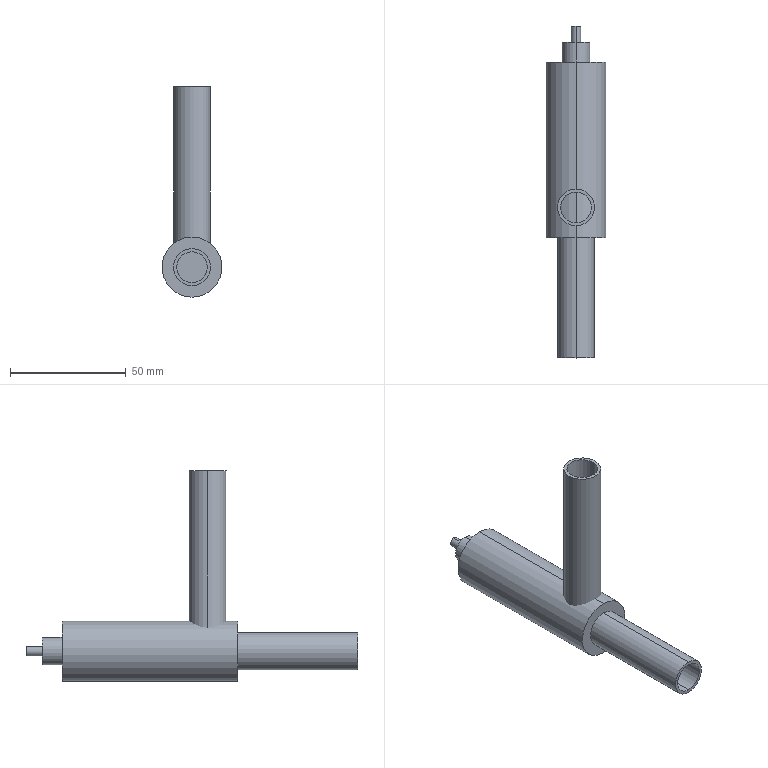Part | STEP file | DX3-012-electronic expansion valve | 3 solids | 22 faces | box 26 x 143.6 x 91 mm | volume 49456 mm3 | cylinder 14 | plane 8 | commonest cylinder face diameters 13.3 x4 16 x4 4 x2 11.8 x2 26 x2
STEP:
#1=CARTESIAN_POINT('',(0.,0.,0.));
#2=DIRECTION('',(0.,0.,1.));
#3=DIRECTION('',(1.,0.,0.));
#4=AXIS2_PLACEMENT_3D('',#1,#2,#3);
#5=CARTESIAN_POINT('',(-8.,13.,78.));
#6=VERTEX_POINT('',#5);
#7=CARTESIAN_POINT('',(8.,13.,78.));
#8=VERTEX_POINT('',#7);
#9=CARTESIAN_POINT('',(0.,13.,78.));
#10=DIRECTION('',(0.,0.,-1.));
#11=DIRECTION('',(-1.,0.,0.));
#12=AXIS2_PLACEMENT_3D('',#9,#10,#11);
#13=CIRCLE('',#12,8.);
#14=CARTESIAN_POINT('',(0.,13.,78.));
#15=DIRECTION('',(0.,0.,-1.));
#16=DIRECTION('',(-1.,0.,0.));
#17=AXIS2_PLACEMENT_3D('',#14,#15,#16);
#18=CYLINDRICAL_SURFACE('',#17,8.);
#19=CARTESIAN_POINT('',(0.,0.));
#20=DIRECTION('',(1.,0.));
#21=VECTOR('',#20,1.);
#22=LINE('',#19,#21);
#23=(GEOMETRIC_REPRESENTATION_CONTEXT(2)PARAMETRIC_REPRESENTATION_CONTEXT()REPRESENTATION_CONTEXT('',''));
#24=DEFINITIONAL_REPRESENTATION('',(#22),#23);
#25=PCURVE('',#18,#24);
#26=CARTESIAN_POINT('',(0.,13.,78.));
#27=DIRECTION('',(0.,0.,1.));
#28=DIRECTION('',(1.,0.,0.));
#29=AXIS2_PLACEMENT_3D('',#26,#27,#28);
#30=PLANE('',#29);
#31=CARTESIAN_POINT('',(-8.,0.));
#32=CARTESIAN_POINT('',(-8.,13.856));
#33=CARTESIAN_POINT('',(4.,6.928));
#34=CARTESIAN_POINT('',(16.,0.));
#35=CARTESIAN_POINT('',(4.,-6.928));
#36=CARTESIAN_POINT('',(-8.,-13.856));
#37=CARTESIAN_POINT('',(-8.,0.));
#38=(BOUNDED_CURVE()B_SPLINE_CURVE(2,(#31,#32,#33,#34,#35,#36,#37),.UNSPECIFIED.,.T.,.F.)B_SPLINE_CURVE_WITH_KNOTS((1,2,2,2,2,1),(-2.094,0.,2.094,4.189,6.283,8.378),.UNSPECIFIED.)CURVE()GEOMETRIC_REPRESENTATION_ITEM()RATIONAL_B_SPLINE_CURVE((1.,0.5,1.,0.5,1.,0.5,1.))REPRESENTATION_ITEM(''));
#39=(GEOMETRIC_REPRESENTATION_CONTEXT(2)PARAMETRIC_REPRESENTATION_CONTEXT()REPRESENTATION_CONTEXT('',''));
#40=DEFINITIONAL_REPRESENTATION('',(#38),#39);
#41=PCURVE('',#30,#40);
#42=SURFACE_CURVE('',#13,(#25,#41),.PCURVE_S1.);
#43=EDGE_CURVE('',#6,#8,#42,.T.);
#44=ORIENTED_EDGE('',*,*,#43,.T.);
#45=CARTESIAN_POINT('',(8.,13.,0.));
#46=VERTEX_POINT('',#45);
#47=CARTESIAN_POINT('',(8.,13.,78.));
#48=DIRECTION('',(0.,0.,-1.));
#49=VECTOR('',#48,1.);
#50=LINE('',#47,#49);
#51=CARTESIAN_POINT('',(3.142,0.));
#52=DIRECTION('',(0.,1.));
#53=VECTOR('',#52,1.);
#54=LINE('',#51,#53);
#55=(GEOMETRIC_REPRESENTATION_CONTEXT(2)PARAMETRIC_REPRESENTATION_CONTEXT()REPRESENTATION_CONTEXT('',''));
#56=DEFINITIONAL_REPRESENTATION('',(#54),#55);
#57=PCURVE('',#18,#56);
#58=CARTESIAN_POINT('',(0.,13.,78.));
#59=DIRECTION('',(0.,0.,-1.));
#60=DIRECTION('',(-1.,0.,0.));
#61=AXIS2_PLACEMENT_3D('',#58,#59,#60);
#62=CYLINDRICAL_SURFACE('',#61,8.);
#63=CARTESIAN_POINT('',(3.142,0.));
#64=DIRECTION('',(0.,1.));
#65=VECTOR('',#64,1.);
#66=LINE('',#63,#65);
#67=(GEOMETRIC_REPRESENTATION_CONTEXT(2)PARAMETRIC_REPRESENTATION_CONTEXT()REPRESENTATION_CONTEXT('',''));
#68=DEFINITIONAL_REPRESENTATION('',(#66),#67);
#69=PCURVE('',#62,#68);
#70=SURFACE_CURVE('',#50,(#57,#69),.PCURVE_S1.);
#71=EDGE_CURVE('',#8,#46,#70,.T.);
#72=ORIENTED_EDGE('',*,*,#71,.T.);
#73=CARTESIAN_POINT('',(-8.,13.,0.));
#74=VERTEX_POINT('',#73);
#75=CARTESIAN_POINT('',(0.,13.,0.));
#76=DIRECTION('',(0.,0.,1.));
#77=DIRECTION('',(-1.,0.,0.));
#78=AXIS2_PLACEMENT_3D('',#75,#76,#77);
#79=CIRCLE('',#78,8.);
#80=CARTESIAN_POINT('',(6.283,78.));
#81=DIRECTION('',(-1.,0.));
#82=VECTOR('',#81,1.);
#83=LINE('',#80,#82);
#84=(GEOMETRIC_REPRESENTATION_CONTEXT(2)PARAMETRIC_REPRESENTATION_CONTEXT()REPRESENTATION_CONTEXT('',''));
#85=DEFINITIONAL_REPRESENTATION('',(#83),#84);
#86=PCURVE('',#18,#85);
#87=CARTESIAN_POINT('',(0.,13.,0.));
#88=DIRECTION('',(0.,0.,1.));
#89=DIRECTION('',(1.,0.,0.));
#90=AXIS2_PLACEMENT_3D('',#87,#88,#89);
#91=PLANE('',#90);
#92=CARTESIAN_POINT('',(0.,0.));
#93=DIRECTION('',(-1.,0.));
#94=AXIS2_PLACEMENT_2D('',#92,#93);
#95=CIRCLE('',#94,8.);
#96=(GEOMETRIC_REPRESENTATION_CONTEXT(2)PARAMETRIC_REPRESENTATION_CONTEXT()REPRESENTATION_CONTEXT('',''));
#97=DEFINITIONAL_REPRESENTATION('',(#95),#96);
#98=PCURVE('',#91,#97);
#99=SURFACE_CURVE('',#79,(#86,#98),.PCURVE_S1.);
#100=EDGE_CURVE('',#46,#74,#99,.T.);
#101=ORIENTED_EDGE('',*,*,#100,.T.);
#102=CARTESIAN_POINT('',(-8.,13.,78.));
#103=DIRECTION('',(0.,0.,-1.));
#104=VECTOR('',#103,1.);
#105=LINE('',#102,#104);
#106=CARTESIAN_POINT('',(0.,0.));
#107=DIRECTION('',(0.,1.));
#108=VECTOR('',#107,1.);
#109=LINE('',#106,#108);
#110=(GEOMETRIC_REPRESENTATION_CONTEXT(2)PARAMETRIC_REPRESENTATION_CONTEXT()REPRESENTATION_CONTEXT('',''));
#111=DEFINITIONAL_REPRESENTATION('',(#109),#110);
#112=PCURVE('',#18,#111);
#113=CARTESIAN_POINT('',(6.283,0.));
#114=DIRECTION('',(0.,1.));
#115=VECTOR('',#114,1.);
#116=LINE('',#113,#115);
#117=(GEOMETRIC_REPRESENTATION_CONTEXT(2)PARAMETRIC_REPRESENTATION_CONTEXT()REPRESENTATION_CONTEXT('',''));
#118=DEFINITIONAL_REPRESENTATION('',(#116),#117);
#119=PCURVE('',#62,#118);
#120=SURFACE_CURVE('',#105,(#112,#119),.PCURVE_S1.);
#121=EDGE_CURVE('',#6,#74,#120,.T.);
#122=ORIENTED_EDGE('',*,*,#121,.F.);
#123=EDGE_LOOP('',(#44,#72,#101,#122));
#124=FACE_BOUND('',#123,.T.);
#125=ADVANCED_FACE('',(#124),#18,.T.);
#126=CARTESIAN_POINT('',(-6.65,13.,78.));
#127=VERTEX_POINT('',#126);
#128=CARTESIAN_POINT('',(-6.65,13.,0.));
#129=VERTEX_POINT('',#128);
#130=CARTESIAN_POINT('',(-6.65,13.,78.));
#131=DIRECTION('',(0.,0.,-1.));
#132=VECTOR('',#131,1.);
#133=LINE('',#130,#132);
#134=CARTESIAN_POINT('',(0.,13.,78.));
#135=DIRECTION('',(0.,0.,-1.));
#136=DIRECTION('',(-1.,0.,0.));
#137=AXIS2_PLACEMENT_3D('',#134,#135,#136);
#138=CYLINDRICAL_SURFACE('',#137,6.65);
#139=CARTESIAN_POINT('',(6.283,0.));
#140=DIRECTION('',(0.,1.));
#141=VECTOR('',#140,1.);
#142=LINE('',#139,#141);
#143=(GEOMETRIC_REPRESENTATION_CONTEXT(2)PARAMETRIC_REPRESENTATION_CONTEXT()REPRESENTATION_CONTEXT('',''));
#144=DEFINITIONAL_REPRESENTATION('',(#142),#143);
#145=PCURVE('',#138,#144);
#146=CARTESIAN_POINT('',(0.,13.,78.));
#147=DIRECTION('',(0.,0.,-1.));
#148=DIRECTION('',(-1.,0.,0.));
#149=AXIS2_PLACEMENT_3D('',#146,#147,#148);
#150=CYLINDRICAL_SURFACE('',#149,6.65);
#151=CARTESIAN_POINT('',(0.,0.));
#152=DIRECTION('',(0.,1.));
#153=VECTOR('',#152,1.);
#154=LINE('',#151,#153);
#155=(GEOMETRIC_REPRESENTATION_CONTEXT(2)PARAMETRIC_REPRESENTATION_CONTEXT()REPRESENTATION_CONTEXT('',''));
#156=DEFINITIONAL_REPRESENTATION('',(#154),#155);
#157=PCURVE('',#150,#156);
#158=SURFACE_CURVE('',#133,(#145,#157),.PCURVE_S1.);
#159=EDGE_CURVE('',#127,#129,#158,.T.);
#160=ORIENTED_EDGE('',*,*,#159,.T.);
#161=CARTESIAN_POINT('',(6.65,13.,0.));
#162=VERTEX_POINT('',#161);
#163=CARTESIAN_POINT('',(0.,13.,0.));
#164=DIRECTION('',(0.,0.,-1.));
#165=DIRECTION('',(-1.,0.,0.));
#166=AXIS2_PLACEMENT_3D('',#163,#164,#165);
#167=CIRCLE('',#166,6.65);
#168=CARTESIAN_POINT('',(0.,78.));
#169=DIRECTION('',(1.,0.));
#170=VECTOR('',#169,1.);
#171=LINE('',#168,#170);
#172=(GEOMETRIC_REPRESENTATION_CONTEXT(2)PARAMETRIC_REPRESENTATION_CONTEXT()REPRESENTATION_CONTEXT('',''));
#173=DEFINITIONAL_REPRESENTATION('',(#171),#172);
#174=PCURVE('',#138,#173);
#175=CARTESIAN_POINT('',(-6.65,0.));
#176=CARTESIAN_POINT('',(-6.65,11.518));
#177=CARTESIAN_POINT('',(3.325,5.759));
#178=CARTESIAN_POINT('',(13.3,0.));
#179=CARTESIAN_POINT('',(3.325,-5.759));
#180=CARTESIAN_POINT('',(-6.65,-11.518));
#181=CARTESIAN_POINT('',(-6.65,0.));
#182=(BOUNDED_CURVE()B_SPLINE_CURVE(2,(#175,#176,#177,#178,#179,#180,#181),.UNSPECIFIED.,.T.,.F.)B_SPLINE_CURVE_WITH_KNOTS((1,2,2,2,2,1),(-2.094,0.,2.094,4.189,6.283,8.378),.UNSPECIFIED.)CURVE()GEOMETRIC_REPRESENTATION_ITEM()RATIONAL_B_SPLINE_CURVE((1.,0.5,1.,0.5,1.,0.5,1.))REPRESENTATION_ITEM(''));
#183=(GEOMETRIC_REPRESENTATION_CONTEXT(2)PARAMETRIC_REPRESENTATION_CONTEXT()REPRESENTATION_CONTEXT('',''));
#184=DEFINITIONAL_REPRESENTATION('',(#182),#183);
#185=PCURVE('',#91,#184);
#186=SURFACE_CURVE('',#167,(#174,#185),.PCURVE_S1.);
#187=EDGE_CURVE('',#162,#129,#186,.T.);
#188=ORIENTED_EDGE('',*,*,#187,.F.);
#189=CARTESIAN_POINT('',(6.65,13.,78.));
#190=VERTEX_POINT('',#189);
#191=CARTESIAN_POINT('',(6.65,13.,78.));
#192=DIRECTION('',(0.,0.,-1.));
#193=VECTOR('',#192,1.);
#194=LINE('',#191,#193);
#195=CARTESIAN_POINT('',(3.142,0.));
#196=DIRECTION('',(0.,1.));
#197=VECTOR('',#196,1.);
#198=LINE('',#195,#197);
#199=(GEOMETRIC_REPRESENTATION_CONTEXT(2)PARAMETRIC_REPRESENTATION_CONTEXT()REPRESENTATION_CONTEXT('',''));
#200=DEFINITIONAL_REPRESENTATION('',(#198),#199);
#201=PCURVE('',#138,#200);
#202=CARTESIAN_POINT('',(3.142,0.));
#203=DIRECTION('',(0.,1.));
#204=VECTOR('',#203,1.);
#205=LINE('',#202,#204);
#206=(GEOMETRIC_REPRESENTATION_CONTEXT(2)PARAMETRIC_REPRESENTATION_CONTEXT()REPRESENTATION_CONTEXT('',''));
#207=DEFINITIONAL_REPRESENTATION('',(#205),#206);
#208=PCURVE('',#150,#207);
#209=SURFACE_CURVE('',#194,(#201,#208),.PCURVE_S1.);
#210=EDGE_CURVE('',#190,#162,#209,.T.);
#211=ORIENTED_EDGE('',*,*,#210,.F.);
#212=CARTESIAN_POINT('',(0.,13.,78.));
#213=DIRECTION('',(0.,0.,-1.));
#214=DIRECTION('',(-1.,0.,0.));
#215=AXIS2_PLACEMENT_3D('',#212,#213,#214);
#216=CIRCLE('',#215,6.65);
#217=CARTESIAN_POINT('',(0.,0.));
#218=DIRECTION('',(1.,0.));
#219=VECTOR('',#218,1.);
#220=LINE('',#217,#219);
#221=(GEOMETRIC_REPRESENTATION_CONTEXT(2)PARAMETRIC_REPRESENTATION_CONTEXT()REPRESENTATION_CONTEXT('',''));
#222=DEFINITIONAL_REPRESENTATION('',(#220),#221);
#223=PCURVE('',#138,#222);
#224=CARTESIAN_POINT('',(-6.65,0.));
#225=CARTESIAN_POINT('',(-6.65,11.518));
#226=CARTESIAN_POINT('',(3.325,5.759));
#227=CARTESIAN_POINT('',(13.3,0.));
#228=CARTESIAN_POINT('',(3.325,-5.759));
#229=CARTESIAN_POINT('',(-6.65,-11.518));
#230=CARTESIAN_POINT('',(-6.65,0.));
#231=(BOUNDED_CURVE()B_SPLINE_CURVE(2,(#224,#225,#226,#227,#228,#229,#230),.UNSPECIFIED.,.T.,.F.)B_SPLINE_CURVE_WITH_KNOTS((1,2,2,2,2,1),(-2.094,0.,2.094,4.189,6.283,8.378),.UNSPECIFIED.)CURVE()GEOMETRIC_REPRESENTATION_ITEM()RATIONAL_B_SPLINE_CURVE((1.,0.5,1.,0.5,1.,0.5,1.))REPRESENTATION_ITEM(''));
#232=(GEOMETRIC_REPRESENTATION_CONTEXT(2)PARAMETRIC_REPRESENTATION_CONTEXT()REPRESENTATION_CONTEXT('',''));
#233=DEFINITIONAL_REPRESENTATION('',(#231),#232);
#234=PCURVE('',#30,#233);
#235=SURFACE_CURVE('',#216,(#223,#234),.PCURVE_S1.);
#236=EDGE_CURVE('',#190,#127,#235,.T.);
#237=ORIENTED_EDGE('',*,*,#236,.T.);
#238=EDGE_LOOP('',(#160,#188,#211,#237));
#239=FACE_BOUND('',#238,.F.);
#240=ADVANCED_FACE('',(#239),#138,.F.);
#241=ORIENTED_EDGE('',*,*,#71,.F.);
#242=CARTESIAN_POINT('',(0.,13.,78.));
#243=DIRECTION('',(0.,0.,-1.));
#244=DIRECTION('',(-1.,0.,0.));
#245=AXIS2_PLACEMENT_3D('',#242,#243,#244);
#246=CIRCLE('',#245,8.);
#247=CARTESIAN_POINT('',(0.,0.));
#248=DIRECTION('',(1.,0.));
#249=VECTOR('',#248,1.);
#250=LINE('',#247,#249);
#251=(GEOMETRIC_REPRESENTATION_CONTEXT(2)PARAMETRIC_REPRESENTATION_CONTEXT()REPRESENTATION_CONTEXT('',''));
#252=DEFINITIONAL_REPRESENTATION('',(#250),#251);
#253=PCURVE('',#62,#252);
#254=CARTESIAN_POINT('',(-8.,0.));
#255=CARTESIAN_POINT('',(-8.,13.856));
#256=CARTESIAN_POINT('',(4.,6.928));
#257=CARTESIAN_POINT('',(16.,0.));
#258=CARTESIAN_POINT('',(4.,-6.928));
#259=CARTESIAN_POINT('',(-8.,-13.856));
#260=CARTESIAN_POINT('',(-8.,0.));
#261=(BOUNDED_CURVE()B_SPLINE_CURVE(2,(#254,#255,#256,#257,#258,#259,#260),.UNSPECIFIED.,.T.,.F.)B_SPLINE_CURVE_WITH_KNOTS((1,2,2,2,2,1),(-2.094,0.,2.094,4.189,6.283,8.378),.UNSPECIFIED.)CURVE()GEOMETRIC_REPRESENTATION_ITEM()RATIONAL_B_SPLINE_CURVE((1.,0.5,1.,0.5,1.,0.5,1.))REPRESENTATION_ITEM(''));
#262=(GEOMETRIC_REPRESENTATION_CONTEXT(2)PARAMETRIC_REPRESENTATION_CONTEXT()REPRESENTATION_CONTEXT('',''));
#263=DEFINITIONAL_REPRESENTATION('',(#261),#262);
#264=PCURVE('',#30,#263);
#265=SURFACE_CURVE('',#246,(#253,#264),.PCURVE_S1.);
#266=EDGE_CURVE('',#8,#6,#265,.T.);
#267=ORIENTED_EDGE('',*,*,#266,.T.);
#268=ORIENTED_EDGE('',*,*,#121,.T.);
#269=CARTESIAN_POINT('',(0.,13.,0.));
#270=DIRECTION('',(0.,0.,1.));
#271=DIRECTION('',(-1.,0.,0.));
#272=AXIS2_PLACEMENT_3D('',#269,#270,#271);
#273=CIRCLE('',#272,8.);
#274=CARTESIAN_POINT('',(6.283,78.));
#275=DIRECTION('',(-1.,0.));
#276=VECTOR('',#275,1.);
#277=LINE('',#274,#276);
#278=(GEOMETRIC_REPRESENTATION_CONTEXT(2)PARAMETRIC_REPRESENTATION_CONTEXT()REPRESENTATION_CONTEXT('',''));
#279=DEFINITIONAL_REPRESENTATION('',(#277),#278);
#280=PCURVE('',#62,#279);
#281=CARTESIAN_POINT('',(0.,0.));
#282=DIRECTION('',(-1.,0.));
#283=AXIS2_PLACEMENT_2D('',#281,#282);
#284=CIRCLE('',#283,8.);
#285=(GEOMETRIC_REPRESENTATION_CONTEXT(2)PARAMETRIC_REPRESENTATION_CONTEXT()REPRESENTATION_CONTEXT('',''));
#286=DEFINITIONAL_REPRESENTATION('',(#284),#285);
#287=PCURVE('',#91,#286);
#288=SURFACE_CURVE('',#273,(#280,#287),.PCURVE_S1.);
#289=EDGE_CURVE('',#74,#46,#288,.T.);
#290=ORIENTED_EDGE('',*,*,#289,.T.);
#291=EDGE_LOOP('',(#241,#267,#268,#290));
#292=FACE_BOUND('',#291,.T.);
#293=ADVANCED_FACE('',(#292),#62,.T.);
#294=CARTESIAN_POINT('',(0.,13.,0.));
#295=DIRECTION('',(0.,0.,-1.));
#296=DIRECTION('',(-1.,0.,0.));
#297=AXIS2_PLACEMENT_3D('',#294,#295,#296);
#298=CIRCLE('',#297,6.65);
#299=CARTESIAN_POINT('',(-6.65,0.));
#300=CARTESIAN_POINT('',(-6.65,11.518));
#301=CARTESIAN_POINT('',(3.325,5.759));
#302=CARTESIAN_POINT('',(13.3,0.));
#303=CARTESIAN_POINT('',(3.325,-5.759));
#304=CARTESIAN_POINT('',(-6.65,-11.518));
#305=CARTESIAN_POINT('',(-6.65,0.));
#306=(BOUNDED_CURVE()B_SPLINE_CURVE(2,(#299,#300,#301,#302,#303,#304,#305),.UNSPECIFIED.,.T.,.F.)B_SPLINE_CURVE_WITH_KNOTS((1,2,2,2,2,1),(-2.094,0.,2.094,4.189,6.283,8.378),.UNSPECIFIED.)CURVE()GEOMETRIC_REPRESENTATION_ITEM()RATIONAL_B_SPLINE_CURVE((1.,0.5,1.,0.5,1.,0.5,1.))REPRESENTATION_ITEM(''));
#307=(GEOMETRIC_REPRESENTATION_CONTEXT(2)PARAMETRIC_REPRESENTATION_CONTEXT()REPRESENTATION_CONTEXT('',''));
#308=DEFINITIONAL_REPRESENTATION('',(#306),#307);
#309=PCURVE('',#91,#308);
#310=CARTESIAN_POINT('',(0.,78.));
#311=DIRECTION('',(1.,0.));
#312=VECTOR('',#311,1.);
#313=LINE('',#310,#312);
#314=(GEOMETRIC_REPRESENTATION_CONTEXT(2)PARAMETRIC_REPRESENTATION_CONTEXT()REPRESENTATION_CONTEXT('',''));
#315=DEFINITIONAL_REPRESENTATION('',(#313),#314);
#316=PCURVE('',#150,#315);
#317=SURFACE_CURVE('',#298,(#309,#316),.PCURVE_S1.);
#318=EDGE_CURVE('',#129,#162,#317,.T.);
#319=ORIENTED_EDGE('',*,*,#318,.F.);
#320=ORIENTED_EDGE('',*,*,#187,.F.);
#321=EDGE_LOOP('',(#319,#320));
#322=FACE_BOUND('',#321,.T.);
#323=ORIENTED_EDGE('',*,*,#289,.F.);
#324=ORIENTED_EDGE('',*,*,#100,.F.);
#325=EDGE_LOOP('',(#323,#324));
#326=FACE_BOUND('',#325,.T.);
#327=ADVANCED_FACE('',(#322,#326),#91,.F.);
#328=CARTESIAN_POINT('',(0.,13.,78.));
#329=DIRECTION('',(0.,0.,-1.));
#330=DIRECTION('',(-1.,0.,0.));
#331=AXIS2_PLACEMENT_3D('',#328,#329,#330);
#332=CIRCLE('',#331,6.65);
#333=CARTESIAN_POINT('',(-6.65,0.));
#334=CARTESIAN_POINT('',(-6.65,11.518));
#335=CARTESIAN_POINT('',(3.325,5.759));
#336=CARTESIAN_POINT('',(13.3,0.));
#337=CARTESIAN_POINT('',(3.325,-5.759));
#338=CARTESIAN_POINT('',(-6.65,-11.518));
#339=CARTESIAN_POINT('',(-6.65,0.));
#340=(BOUNDED_CURVE()B_SPLINE_CURVE(2,(#333,#334,#335,#336,#337,#338,#339),.UNSPECIFIED.,.T.,.F.)B_SPLINE_CURVE_WITH_KNOTS((1,2,2,2,2,1),(-2.094,0.,2.094,4.189,6.283,8.378),.UNSPECIFIED.)CURVE()GEOMETRIC_REPRESENTATION_ITEM()RATIONAL_B_SPLINE_CURVE((1.,0.5,1.,0.5,1.,0.5,1.))REPRESENTATION_ITEM(''));
#341=(GEOMETRIC_REPRESENTATION_CONTEXT(2)PARAMETRIC_REPRESENTATION_CONTEXT()REPRESENTATION_CONTEXT('',''));
#342=DEFINITIONAL_REPRESENTATION('',(#340),#341);
#343=PCURVE('',#30,#342);
#344=CARTESIAN_POINT('',(0.,0.));
#345=DIRECTION('',(1.,0.));
#346=VECTOR('',#345,1.);
#347=LINE('',#344,#346);
#348=(GEOMETRIC_REPRESENTATION_CONTEXT(2)PARAMETRIC_REPRESENTATION_CONTEXT()REPRESENTATION_CONTEXT('',''));
#349=DEFINITIONAL_REPRESENTATION('',(#347),#348);
#350=PCURVE('',#150,#349);
#351=SURFACE_CURVE('',#332,(#343,#350),.PCURVE_S1.);
#352=EDGE_CURVE('',#127,#190,#351,.T.);
#353=ORIENTED_EDGE('',*,*,#352,.T.);
#354=ORIENTED_EDGE('',*,*,#236,.T.);
#355=EDGE_LOOP('',(#353,#354));
#356=FACE_BOUND('',#355,.T.);
#357=ORIENTED_EDGE('',*,*,#43,.F.);
#358=ORIENTED_EDGE('',*,*,#266,.F.);
#359=EDGE_LOOP('',(#357,#358));
#360=FACE_BOUND('',#359,.T.);
#361=ADVANCED_FACE('',(#356,#360),#30,.T.);
#362=ORIENTED_EDGE('',*,*,#318,.F.);
#363=ORIENTED_EDGE('',*,*,#159,.F.);
#364=ORIENTED_EDGE('',*,*,#352,.T.);
#365=ORIENTED_EDGE('',*,*,#210,.T.);
#366=EDGE_LOOP('',(#362,#363,#364,#365));
#367=FACE_BOUND('',#366,.F.);
#368=ADVANCED_FACE('',(#367),#150,.F.);
#369=CLOSED_SHELL('',(#125,#240,#293,#327,#361,#368));
#370=MANIFOLD_SOLID_BREP('',#369);
#371=CARTESIAN_POINT('',(0.,76.,-13.));
#372=VERTEX_POINT('',#371);
#373=CARTESIAN_POINT('',(0.,76.,13.));
#374=VERTEX_POINT('',#373);
#375=CARTESIAN_POINT('',(0.,76.,0.));
#376=DIRECTION('',(0.,-1.,0.));
#377=DIRECTION('',(0.,0.,-1.));
#378=AXIS2_PLACEMENT_3D('',#375,#376,#377);
#379=CIRCLE('',#378,13.);
#380=CARTESIAN_POINT('',(0.,76.,0.));
#381=DIRECTION('',(0.,-1.,0.));
#382=DIRECTION('',(0.,0.,-1.));
#383=AXIS2_PLACEMENT_3D('',#380,#381,#382);
#384=CYLINDRICAL_SURFACE('',#383,13.);
#385=CARTESIAN_POINT('',(0.,0.));
#386=DIRECTION('',(1.,0.));
#387=VECTOR('',#386,1.);
#388=LINE('',#385,#387);
#389=(GEOMETRIC_REPRESENTATION_CONTEXT(2)PARAMETRIC_REPRESENTATION_CONTEXT()REPRESENTATION_CONTEXT('',''));
#390=DEFINITIONAL_REPRESENTATION('',(#388),#389);
#391=PCURVE('',#384,#390);
#392=CARTESIAN_POINT('',(0.,76.,0.));
#393=DIRECTION('',(0.,1.,0.));
#394=DIRECTION('',(0.,0.,1.));
#395=AXIS2_PLACEMENT_3D('',#392,#393,#394);
#396=PLANE('',#395);
#397=CARTESIAN_POINT('',(-13.,0.));
#398=CARTESIAN_POINT('',(-13.,22.517));
#399=CARTESIAN_POINT('',(6.5,11.258));
#400=CARTESIAN_POINT('',(26.,0.));
#401=CARTESIAN_POINT('',(6.5,-11.258));
#402=CARTESIAN_POINT('',(-13.,-22.517));
#403=CARTESIAN_POINT('',(-13.,0.));
#404=(BOUNDED_CURVE()B_SPLINE_CURVE(2,(#397,#398,#399,#400,#401,#402,#403),.UNSPECIFIED.,.T.,.F.)B_SPLINE_CURVE_WITH_KNOTS((1,2,2,2,2,1),(-2.094,0.,2.094,4.189,6.283,8.378),.UNSPECIFIED.)CURVE()GEOMETRIC_REPRESENTATION_ITEM()RATIONAL_B_SPLINE_CURVE((1.,0.5,1.,0.5,1.,0.5,1.))REPRESENTATION_ITEM(''));
#405=(GEOMETRIC_REPRESENTATION_CONTEXT(2)PARAMETRIC_REPRESENTATION_CONTEXT()REPRESENTATION_CONTEXT('',''));
#406=DEFINITIONAL_REPRESENTATION('',(#404),#405);
#407=PCURVE('',#396,#406);
#408=SURFACE_CURVE('',#379,(#391,#407),.PCURVE_S1.);
#409=EDGE_CURVE('',#372,#374,#408,.T.);
#410=ORIENTED_EDGE('',*,*,#409,.T.);
#411=CARTESIAN_POINT('',(0.,0.,13.));
#412=VERTEX_POINT('',#411);
#413=CARTESIAN_POINT('',(0.,76.,13.));
#414=DIRECTION('',(0.,-1.,0.));
#415=VECTOR('',#414,1.);
#416=LINE('',#413,#415);
#417=CARTESIAN_POINT('',(3.142,0.));
#418=DIRECTION('',(0.,1.));
#419=VECTOR('',#418,1.);
#420=LINE('',#417,#419);
#421=(GEOMETRIC_REPRESENTATION_CONTEXT(2)PARAMETRIC_REPRESENTATION_CONTEXT()REPRESENTATION_CONTEXT('',''));
#422=DEFINITIONAL_REPRESENTATION('',(#420),#421);
#423=PCURVE('',#384,#422);
#424=CARTESIAN_POINT('',(0.,76.,0.));
#425=DIRECTION('',(0.,-1.,0.));
#426=DIRECTION('',(0.,0.,-1.));
#427=AXIS2_PLACEMENT_3D('',#424,#425,#426);
#428=CYLINDRICAL_SURFACE('',#427,13.);
#429=CARTESIAN_POINT('',(3.142,0.));
#430=DIRECTION('',(0.,1.));
#431=VECTOR('',#430,1.);
#432=LINE('',#429,#431);
#433=(GEOMETRIC_REPRESENTATION_CONTEXT(2)PARAMETRIC_REPRESENTATION_CONTEXT()REPRESENTATION_CONTEXT('',''));
#434=DEFINITIONAL_REPRESENTATION('',(#432),#433);
#435=PCURVE('',#428,#434);
#436=SURFACE_CURVE('',#416,(#423,#435),.PCURVE_S1.);
#437=EDGE_CURVE('',#374,#412,#436,.T.);
#438=ORIENTED_EDGE('',*,*,#437,.T.);
#439=CARTESIAN_POINT('',(0.,0.,-13.));
#440=VERTEX_POINT('',#439);
#441=CARTESIAN_POINT('',(0.,0.,0.));
#442=DIRECTION('',(0.,1.,0.));
#443=DIRECTION('',(0.,0.,-1.));
#444=AXIS2_PLACEMENT_3D('',#441,#442,#443);
#445=CIRCLE('',#444,13.);
#446=CARTESIAN_POINT('',(6.283,76.));
#447=DIRECTION('',(-1.,0.));
#448=VECTOR('',#447,1.);
#449=LINE('',#446,#448);
#450=(GEOMETRIC_REPRESENTATION_CONTEXT(2)PARAMETRIC_REPRESENTATION_CONTEXT()REPRESENTATION_CONTEXT('',''));
#451=DEFINITIONAL_REPRESENTATION('',(#449),#450);
#452=PCURVE('',#384,#451);
#453=CARTESIAN_POINT('',(0.,0.,0.));
#454=DIRECTION('',(0.,1.,0.));
#455=DIRECTION('',(0.,0.,1.));
#456=AXIS2_PLACEMENT_3D('',#453,#454,#455);
#457=PLANE('',#456);
#458=CARTESIAN_POINT('',(0.,0.));
#459=DIRECTION('',(-1.,0.));
#460=AXIS2_PLACEMENT_2D('',#458,#459);
#461=CIRCLE('',#460,13.);
#462=(GEOMETRIC_REPRESENTATION_CONTEXT(2)PARAMETRIC_REPRESENTATION_CONTEXT()REPRESENTATION_CONTEXT('',''));
#463=DEFINITIONAL_REPRESENTATION('',(#461),#462);
#464=PCURVE('',#457,#463);
#465=SURFACE_CURVE('',#445,(#452,#464),.PCURVE_S1.);
#466=EDGE_CURVE('',#412,#440,#465,.T.);
#467=ORIENTED_EDGE('',*,*,#466,.T.);
#468=CARTESIAN_POINT('',(0.,76.,-13.));
#469=DIRECTION('',(0.,-1.,0.));
#470=VECTOR('',#469,1.);
#471=LINE('',#468,#470);
#472=CARTESIAN_POINT('',(0.,0.));
#473=DIRECTION('',(0.,1.));
#474=VECTOR('',#473,1.);
#475=LINE('',#472,#474);
#476=(GEOMETRIC_REPRESENTATION_CONTEXT(2)PARAMETRIC_REPRESENTATION_CONTEXT()REPRESENTATION_CONTEXT('',''));
#477=DEFINITIONAL_REPRESENTATION('',(#475),#476);
#478=PCURVE('',#384,#477);
#479=CARTESIAN_POINT('',(6.283,0.));
#480=DIRECTION('',(0.,1.));
#481=VECTOR('',#480,1.);
#482=LINE('',#479,#481);
#483=(GEOMETRIC_REPRESENTATION_CONTEXT(2)PARAMETRIC_REPRESENTATION_CONTEXT()REPRESENTATION_CONTEXT('',''));
#484=DEFINITIONAL_REPRESENTATION('',(#482),#483);
#485=PCURVE('',#428,#484);
#486=SURFACE_CURVE('',#471,(#478,#485),.PCURVE_S1.);
#487=EDGE_CURVE('',#372,#440,#486,.T.);
#488=ORIENTED_EDGE('',*,*,#487,.F.);
#489=EDGE_LOOP('',(#410,#438,#467,#488));
#490=FACE_BOUND('',#489,.T.);
#491=ADVANCED_FACE('',(#490),#384,.T.);
#492=CARTESIAN_POINT('',(0.,84.6,-5.9));
#493=VERTEX_POINT('',#492);
#494=CARTESIAN_POINT('',(0.,84.6,5.9));
#495=VERTEX_POINT('',#494);
#496=CARTESIAN_POINT('',(0.,84.6,0.));
#497=DIRECTION('',(0.,-1.,0.));
#498=DIRECTION('',(0.,0.,-1.));
#499=AXIS2_PLACEMENT_3D('',#496,#497,#498);
#500=CIRCLE('',#499,5.9);
#501=CARTESIAN_POINT('',(0.,84.6,0.));
#502=DIRECTION('',(0.,-1.,0.));
#503=DIRECTION('',(0.,0.,-1.));
#504=AXIS2_PLACEMENT_3D('',#501,#502,#503);
#505=CYLINDRICAL_SURFACE('',#504,5.9);
#506=CARTESIAN_POINT('',(0.,0.));
#507=DIRECTION('',(1.,0.));
#508=VECTOR('',#507,1.);
#509=LINE('',#506,#508);
#510=(GEOMETRIC_REPRESENTATION_CONTEXT(2)PARAMETRIC_REPRESENTATION_CONTEXT()REPRESENTATION_CONTEXT('',''));
#511=DEFINITIONAL_REPRESENTATION('',(#509),#510);
#512=PCURVE('',#505,#511);
#513=CARTESIAN_POINT('',(0.,84.6,0.));
#514=DIRECTION('',(0.,1.,0.));
#515=DIRECTION('',(0.,0.,1.));
#516=AXIS2_PLACEMENT_3D('',#513,#514,#515);
#517=PLANE('',#516);
#518=CARTESIAN_POINT('',(-5.9,0.));
#519=CARTESIAN_POINT('',(-5.9,10.219));
#520=CARTESIAN_POINT('',(2.95,5.11));
#521=CARTESIAN_POINT('',(11.8,0.));
#522=CARTESIAN_POINT('',(2.95,-5.11));
#523=CARTESIAN_POINT('',(-5.9,-10.219));
#524=CARTESIAN_POINT('',(-5.9,0.));
#525=(BOUNDED_CURVE()B_SPLINE_CURVE(2,(#518,#519,#520,#521,#522,#523,#524),.UNSPECIFIED.,.T.,.F.)B_SPLINE_CURVE_WITH_KNOTS((1,2,2,2,2,1),(-2.094,0.,2.094,4.189,6.283,8.378),.UNSPECIFIED.)CURVE()GEOMETRIC_REPRESENTATION_ITEM()RATIONAL_B_SPLINE_CURVE((1.,0.5,1.,0.5,1.,0.5,1.))REPRESENTATION_ITEM(''));
#526=(GEOMETRIC_REPRESENTATION_CONTEXT(2)PARAMETRIC_REPRESENTATION_CONTEXT()REPRESENTATION_CONTEXT('',''));
#527=DEFINITIONAL_REPRESENTATION('',(#525),#526);
#528=PCURVE('',#517,#527);
#529=SURFACE_CURVE('',#500,(#512,#528),.PCURVE_S1.);
#530=EDGE_CURVE('',#493,#495,#529,.T.);
#531=ORIENTED_EDGE('',*,*,#530,.T.);
#532=CARTESIAN_POINT('',(0.,76.,5.9));
#533=VERTEX_POINT('',#532);
#534=CARTESIAN_POINT('',(0.,84.6,5.9));
#535=DIRECTION('',(0.,-1.,0.));
#536=VECTOR('',#535,1.);
#537=LINE('',#534,#536);
#538=CARTESIAN_POINT('',(3.142,0.));
#539=DIRECTION('',(0.,1.));
#540=VECTOR('',#539,1.);
#541=LINE('',#538,#540);
#542=(GEOMETRIC_REPRESENTATION_CONTEXT(2)PARAMETRIC_REPRESENTATION_CONTEXT()REPRESENTATION_CONTEXT('',''));
#543=DEFINITIONAL_REPRESENTATION('',(#541),#542);
#544=PCURVE('',#505,#543);
#545=CARTESIAN_POINT('',(0.,84.6,0.));
#546=DIRECTION('',(0.,-1.,0.));
#547=DIRECTION('',(0.,0.,-1.));
#548=AXIS2_PLACEMENT_3D('',#545,#546,#547);
#549=CYLINDRICAL_SURFACE('',#548,5.9);
#550=CARTESIAN_POINT('',(3.142,0.));
#551=DIRECTION('',(0.,1.));
#552=VECTOR('',#551,1.);
#553=LINE('',#550,#552);
#554=(GEOMETRIC_REPRESENTATION_CONTEXT(2)PARAMETRIC_REPRESENTATION_CONTEXT()REPRESENTATION_CONTEXT('',''));
#555=DEFINITIONAL_REPRESENTATION('',(#553),#554);
#556=PCURVE('',#549,#555);
#557=SURFACE_CURVE('',#537,(#544,#556),.PCURVE_S1.);
#558=EDGE_CURVE('',#495,#533,#557,.T.);
#559=ORIENTED_EDGE('',*,*,#558,.T.);
#560=CARTESIAN_POINT('',(0.,76.,-5.9));
#561=VERTEX_POINT('',#560);
#562=CARTESIAN_POINT('',(0.,76.,0.));
#563=DIRECTION('',(0.,-1.,0.));
#564=DIRECTION('',(0.,0.,-1.));
#565=AXIS2_PLACEMENT_3D('',#562,#563,#564);
#566=CIRCLE('',#565,5.9);
#567=CARTESIAN_POINT('',(0.,8.6));
#568=DIRECTION('',(1.,0.));
#569=VECTOR('',#568,1.);
#570=LINE('',#567,#569);
#571=(GEOMETRIC_REPRESENTATION_CONTEXT(2)PARAMETRIC_REPRESENTATION_CONTEXT()REPRESENTATION_CONTEXT('',''));
#572=DEFINITIONAL_REPRESENTATION('',(#570),#571);
#573=PCURVE('',#505,#572);
#574=CARTESIAN_POINT('',(-5.9,0.));
#575=CARTESIAN_POINT('',(-5.9,10.219));
#576=CARTESIAN_POINT('',(2.95,5.11));
#577=CARTESIAN_POINT('',(11.8,0.));
#578=CARTESIAN_POINT('',(2.95,-5.11));
#579=CARTESIAN_POINT('',(-5.9,-10.219));
#580=CARTESIAN_POINT('',(-5.9,0.));
#581=(BOUNDED_CURVE()B_SPLINE_CURVE(2,(#574,#575,#576,#577,#578,#579,#580),.UNSPECIFIED.,.T.,.F.)B_SPLINE_CURVE_WITH_KNOTS((1,2,2,2,2,1),(-2.094,0.,2.094,4.189,6.283,8.378),.UNSPECIFIED.)CURVE()GEOMETRIC_REPRESENTATION_ITEM()RATIONAL_B_SPLINE_CURVE((1.,0.5,1.,0.5,1.,0.5,1.))REPRESENTATION_ITEM(''));
#582=(GEOMETRIC_REPRESENTATION_CONTEXT(2)PARAMETRIC_REPRESENTATION_CONTEXT()REPRESENTATION_CONTEXT('',''));
#583=DEFINITIONAL_REPRESENTATION('',(#581),#582);
#584=PCURVE('',#396,#583);
#585=SURFACE_CURVE('',#566,(#573,#584),.PCURVE_S1.);
#586=EDGE_CURVE('',#561,#533,#585,.T.);
#587=ORIENTED_EDGE('',*,*,#586,.F.);
#588=CARTESIAN_POINT('',(0.,84.6,-5.9));
#589=DIRECTION('',(0.,-1.,0.));
#590=VECTOR('',#589,1.);
#591=LINE('',#588,#590);
#592=CARTESIAN_POINT('',(0.,0.));
#593=DIRECTION('',(0.,1.));
#594=VECTOR('',#593,1.);
#595=LINE('',#592,#594);
#596=(GEOMETRIC_REPRESENTATION_CONTEXT(2)PARAMETRIC_REPRESENTATION_CONTEXT()REPRESENTATION_CONTEXT('',''));
#597=DEFINITIONAL_REPRESENTATION('',(#595),#596);
#598=PCURVE('',#505,#597);
#599=CARTESIAN_POINT('',(6.283,0.));
#600=DIRECTION('',(0.,1.));
#601=VECTOR('',#600,1.);
#602=LINE('',#599,#601);
#603=(GEOMETRIC_REPRESENTATION_CONTEXT(2)PARAMETRIC_REPRESENTATION_CONTEXT()REPRESENTATION_CONTEXT('',''));
#604=DEFINITIONAL_REPRESENTATION('',(#602),#603);
#605=PCURVE('',#549,#604);
#606=SURFACE_CURVE('',#591,(#598,#605),.PCURVE_S1.);
#607=EDGE_CURVE('',#493,#561,#606,.T.);
#608=ORIENTED_EDGE('',*,*,#607,.F.);
#609=EDGE_LOOP('',(#531,#559,#587,#608));
#610=FACE_BOUND('',#609,.T.);
#611=ADVANCED_FACE('',(#610),#505,.T.);
#612=CARTESIAN_POINT('',(0.,91.6,-2.));
#613=VERTEX_POINT('',#612);
#614=CARTESIAN_POINT('',(0.,91.6,2.));
#615=VERTEX_POINT('',#614);
#616=CARTESIAN_POINT('',(0.,91.6,0.));
#617=DIRECTION('',(0.,-1.,0.));
#618=DIRECTION('',(0.,0.,-1.));
#619=AXIS2_PLACEMENT_3D('',#616,#617,#618);
#620=CIRCLE('',#619,2.);
#621=CARTESIAN_POINT('',(0.,91.6,0.));
#622=DIRECTION('',(0.,-1.,0.));
#623=DIRECTION('',(0.,0.,-1.));
#624=AXIS2_PLACEMENT_3D('',#621,#622,#623);
#625=CYLINDRICAL_SURFACE('',#624,2.);
#626=CARTESIAN_POINT('',(0.,0.));
#627=DIRECTION('',(1.,0.));
#628=VECTOR('',#627,1.);
#629=LINE('',#626,#628);
#630=(GEOMETRIC_REPRESENTATION_CONTEXT(2)PARAMETRIC_REPRESENTATION_CONTEXT()REPRESENTATION_CONTEXT('',''));
#631=DEFINITIONAL_REPRESENTATION('',(#629),#630);
#632=PCURVE('',#625,#631);
#633=CARTESIAN_POINT('',(0.,91.6,0.));
#634=DIRECTION('',(0.,1.,0.));
#635=DIRECTION('',(0.,0.,1.));
#636=AXIS2_PLACEMENT_3D('',#633,#634,#635);
#637=PLANE('',#636);
#638=CARTESIAN_POINT('',(-2.,0.));
#639=CARTESIAN_POINT('',(-2.,3.464));
#640=CARTESIAN_POINT('',(1.,1.732));
#641=CARTESIAN_POINT('',(4.,0.));
#642=CARTESIAN_POINT('',(1.,-1.732));
#643=CARTESIAN_POINT('',(-2.,-3.464));
#644=CARTESIAN_POINT('',(-2.,0.));
#645=(BOUNDED_CURVE()B_SPLINE_CURVE(2,(#638,#639,#640,#641,#642,#643,#644),.UNSPECIFIED.,.T.,.F.)B_SPLINE_CURVE_WITH_KNOTS((1,2,2,2,2,1),(-2.094,0.,2.094,4.189,6.283,8.378),.UNSPECIFIED.)CURVE()GEOMETRIC_REPRESENTATION_ITEM()RATIONAL_B_SPLINE_CURVE((1.,0.5,1.,0.5,1.,0.5,1.))REPRESENTATION_ITEM(''));
#646=(GEOMETRIC_REPRESENTATION_CONTEXT(2)PARAMETRIC_REPRESENTATION_CONTEXT()REPRESENTATION_CONTEXT('',''));
#647=DEFINITIONAL_REPRESENTATION('',(#645),#646);
#648=PCURVE('',#637,#647);
#649=SURFACE_CURVE('',#620,(#632,#648),.PCURVE_S1.);
#650=EDGE_CURVE('',#613,#615,#649,.T.);
#651=ORIENTED_EDGE('',*,*,#650,.T.);
#652=CARTESIAN_POINT('',(0.,84.6,2.));
#653=VERTEX_POINT('',#652);
#654=CARTESIAN_POINT('',(0.,91.6,2.));
#655=DIRECTION('',(0.,-1.,0.));
#656=VECTOR('',#655,1.);
#657=LINE('',#654,#656);
#658=CARTESIAN_POINT('',(3.142,0.));
#659=DIRECTION('',(0.,1.));
#660=VECTOR('',#659,1.);
#661=LINE('',#658,#660);
#662=(GEOMETRIC_REPRESENTATION_CONTEXT(2)PARAMETRIC_REPRESENTATION_CONTEXT()REPRESENTATION_CONTEXT('',''));
#663=DEFINITIONAL_REPRESENTATION('',(#661),#662);
#664=PCURVE('',#625,#663);
#665=CARTESIAN_POINT('',(0.,91.6,0.));
#666=DIRECTION('',(0.,-1.,0.));
#667=DIRECTION('',(0.,0.,-1.));
#668=AXIS2_PLACEMENT_3D('',#665,#666,#667);
#669=CYLINDRICAL_SURFACE('',#668,2.);
#670=CARTESIAN_POINT('',(3.142,0.));
#671=DIRECTION('',(0.,1.));
#672=VECTOR('',#671,1.);
#673=LINE('',#670,#672);
#674=(GEOMETRIC_REPRESENTATION_CONTEXT(2)PARAMETRIC_REPRESENTATION_CONTEXT()REPRESENTATION_CONTEXT('',''));
#675=DEFINITIONAL_REPRESENTATION('',(#673),#674);
#676=PCURVE('',#669,#675);
#677=SURFACE_CURVE('',#657,(#664,#676),.PCURVE_S1.);
#678=EDGE_CURVE('',#615,#653,#677,.T.);
#679=ORIENTED_EDGE('',*,*,#678,.T.);
#680=CARTESIAN_POINT('',(0.,84.6,-2.));
#681=VERTEX_POINT('',#680);
#682=CARTESIAN_POINT('',(0.,84.6,0.));
#683=DIRECTION('',(0.,-1.,0.));
#684=DIRECTION('',(0.,0.,-1.));
#685=AXIS2_PLACEMENT_3D('',#682,#683,#684);
#686=CIRCLE('',#685,2.);
#687=CARTESIAN_POINT('',(0.,7.));
#688=DIRECTION('',(1.,0.));
#689=VECTOR('',#688,1.);
#690=LINE('',#687,#689);
#691=(GEOMETRIC_REPRESENTATION_CONTEXT(2)PARAMETRIC_REPRESENTATION_CONTEXT()REPRESENTATION_CONTEXT('',''));
#692=DEFINITIONAL_REPRESENTATION('',(#690),#691);
#693=PCURVE('',#625,#692);
#694=CARTESIAN_POINT('',(-2.,0.));
#695=CARTESIAN_POINT('',(-2.,3.464));
#696=CARTESIAN_POINT('',(1.,1.732));
#697=CARTESIAN_POINT('',(4.,0.));
#698=CARTESIAN_POINT('',(1.,-1.732));
#699=CARTESIAN_POINT('',(-2.,-3.464));
#700=CARTESIAN_POINT('',(-2.,0.));
#701=(BOUNDED_CURVE()B_SPLINE_CURVE(2,(#694,#695,#696,#697,#698,#699,#700),.UNSPECIFIED.,.T.,.F.)B_SPLINE_CURVE_WITH_KNOTS((1,2,2,2,2,1),(-2.094,0.,2.094,4.189,6.283,8.378),.UNSPECIFIED.)CURVE()GEOMETRIC_REPRESENTATION_ITEM()RATIONAL_B_SPLINE_CURVE((1.,0.5,1.,0.5,1.,0.5,1.))REPRESENTATION_ITEM(''));
#702=(GEOMETRIC_REPRESENTATION_CONTEXT(2)PARAMETRIC_REPRESENTATION_CONTEXT()REPRESENTATION_CONTEXT('',''));
#703=DEFINITIONAL_REPRESENTATION('',(#701),#702);
#704=PCURVE('',#517,#703);
#705=SURFACE_CURVE('',#686,(#693,#704),.PCURVE_S1.);
#706=EDGE_CURVE('',#681,#653,#705,.T.);
#707=ORIENTED_EDGE('',*,*,#706,.F.);
#708=CARTESIAN_POINT('',(0.,91.6,-2.));
#709=DIRECTION('',(0.,-1.,0.));
#710=VECTOR('',#709,1.);
#711=LINE('',#708,#710);
#712=CARTESIAN_POINT('',(0.,0.));
#713=DIRECTION('',(0.,1.));
#714=VECTOR('',#713,1.);
#715=LINE('',#712,#714);
#716=(GEOMETRIC_REPRESENTATION_CONTEXT(2)PARAMETRIC_REPRESENTATION_CONTEXT()REPRESENTATION_CONTEXT('',''));
#717=DEFINITIONAL_REPRESENTATION('',(#715),#716);
#718=PCURVE('',#625,#717);
#719=CARTESIAN_POINT('',(6.283,0.));
#720=DIRECTION('',(0.,1.));
#721=VECTOR('',#720,1.);
#722=LINE('',#719,#721);
#723=(GEOMETRIC_REPRESENTATION_CONTEXT(2)PARAMETRIC_REPRESENTATION_CONTEXT()REPRESENTATION_CONTEXT('',''));
#724=DEFINITIONAL_REPRESENTATION('',(#722),#723);
#725=PCURVE('',#669,#724);
#726=SURFACE_CURVE('',#711,(#718,#725),.PCURVE_S1.);
#727=EDGE_CURVE('',#613,#681,#726,.T.);
#728=ORIENTED_EDGE('',*,*,#727,.F.);
#729=EDGE_LOOP('',(#651,#679,#707,#728));
#730=FACE_BOUND('',#729,.T.);
#731=ADVANCED_FACE('',(#730),#625,.T.);
#732=ORIENTED_EDGE('',*,*,#437,.F.);
#733=CARTESIAN_POINT('',(0.,76.,0.));
#734=DIRECTION('',(0.,-1.,0.));
#735=DIRECTION('',(0.,0.,-1.));
#736=AXIS2_PLACEMENT_3D('',#733,#734,#735);
#737=CIRCLE('',#736,13.);
#738=CARTESIAN_POINT('',(0.,0.));
#739=DIRECTION('',(1.,0.));
#740=VECTOR('',#739,1.);
#741=LINE('',#738,#740);
#742=(GEOMETRIC_REPRESENTATION_CONTEXT(2)PARAMETRIC_REPRESENTATION_CONTEXT()REPRESENTATION_CONTEXT('',''));
#743=DEFINITIONAL_REPRESENTATION('',(#741),#742);
#744=PCURVE('',#428,#743);
#745=CARTESIAN_POINT('',(-13.,0.));
#746=CARTESIAN_POINT('',(-13.,22.517));
#747=CARTESIAN_POINT('',(6.5,11.258));
#748=CARTESIAN_POINT('',(26.,0.));
#749=CARTESIAN_POINT('',(6.5,-11.258));
#750=CARTESIAN_POINT('',(-13.,-22.517));
#751=CARTESIAN_POINT('',(-13.,0.));
#752=(BOUNDED_CURVE()B_SPLINE_CURVE(2,(#745,#746,#747,#748,#749,#750,#751),.UNSPECIFIED.,.T.,.F.)B_SPLINE_CURVE_WITH_KNOTS((1,2,2,2,2,1),(-2.094,0.,2.094,4.189,6.283,8.378),.UNSPECIFIED.)CURVE()GEOMETRIC_REPRESENTATION_ITEM()RATIONAL_B_SPLINE_CURVE((1.,0.5,1.,0.5,1.,0.5,1.))REPRESENTATION_ITEM(''));
#753=(GEOMETRIC_REPRESENTATION_CONTEXT(2)PARAMETRIC_REPRESENTATION_CONTEXT()REPRESENTATION_CONTEXT('',''));
#754=DEFINITIONAL_REPRESENTATION('',(#752),#753);
#755=PCURVE('',#396,#754);
#756=SURFACE_CURVE('',#737,(#744,#755),.PCURVE_S1.);
#757=EDGE_CURVE('',#374,#372,#756,.T.);
#758=ORIENTED_EDGE('',*,*,#757,.T.);
#759=ORIENTED_EDGE('',*,*,#487,.T.);
#760=CARTESIAN_POINT('',(0.,0.,0.));
#761=DIRECTION('',(0.,1.,0.));
#762=DIRECTION('',(0.,0.,-1.));
#763=AXIS2_PLACEMENT_3D('',#760,#761,#762);
#764=CIRCLE('',#763,13.);
#765=CARTESIAN_POINT('',(6.283,76.));
#766=DIRECTION('',(-1.,0.));
#767=VECTOR('',#766,1.);
#768=LINE('',#765,#767);
#769=(GEOMETRIC_REPRESENTATION_CONTEXT(2)PARAMETRIC_REPRESENTATION_CONTEXT()REPRESENTATION_CONTEXT('',''));
#770=DEFINITIONAL_REPRESENTATION('',(#768),#769);
#771=PCURVE('',#428,#770);
#772=CARTESIAN_POINT('',(0.,0.));
#773=DIRECTION('',(-1.,0.));
#774=AXIS2_PLACEMENT_2D('',#772,#773);
#775=CIRCLE('',#774,13.);
#776=(GEOMETRIC_REPRESENTATION_CONTEXT(2)PARAMETRIC_REPRESENTATION_CONTEXT()REPRESENTATION_CONTEXT('',''));
#777=DEFINITIONAL_REPRESENTATION('',(#775),#776);
#778=PCURVE('',#457,#777);
#779=SURFACE_CURVE('',#764,(#771,#778),.PCURVE_S1.);
#780=EDGE_CURVE('',#440,#412,#779,.T.);
#781=ORIENTED_EDGE('',*,*,#780,.T.);
#782=EDGE_LOOP('',(#732,#758,#759,#781));
#783=FACE_BOUND('',#782,.T.);
#784=ADVANCED_FACE('',(#783),#428,.T.);
#785=ORIENTED_EDGE('',*,*,#780,.F.);
#786=ORIENTED_EDGE('',*,*,#466,.F.);
#787=EDGE_LOOP('',(#785,#786));
#788=FACE_BOUND('',#787,.T.);
#789=ADVANCED_FACE('',(#788),#457,.F.);
#790=ORIENTED_EDGE('',*,*,#409,.F.);
#791=ORIENTED_EDGE('',*,*,#757,.F.);
#792=EDGE_LOOP('',(#790,#791));
#793=FACE_BOUND('',#792,.T.);
#794=ORIENTED_EDGE('',*,*,#586,.T.);
#795=CARTESIAN_POINT('',(0.,76.,0.));
#796=DIRECTION('',(0.,-1.,0.));
#797=DIRECTION('',(0.,0.,-1.));
#798=AXIS2_PLACEMENT_3D('',#795,#796,#797);
#799=CIRCLE('',#798,5.9);
#800=CARTESIAN_POINT('',(-5.9,0.));
#801=CARTESIAN_POINT('',(-5.9,10.219));
#802=CARTESIAN_POINT('',(2.95,5.11));
#803=CARTESIAN_POINT('',(11.8,0.));
#804=CARTESIAN_POINT('',(2.95,-5.11));
#805=CARTESIAN_POINT('',(-5.9,-10.219));
#806=CARTESIAN_POINT('',(-5.9,0.));
#807=(BOUNDED_CURVE()B_SPLINE_CURVE(2,(#800,#801,#802,#803,#804,#805,#806),.UNSPECIFIED.,.T.,.F.)B_SPLINE_CURVE_WITH_KNOTS((1,2,2,2,2,1),(-2.094,0.,2.094,4.189,6.283,8.378),.UNSPECIFIED.)CURVE()GEOMETRIC_REPRESENTATION_ITEM()RATIONAL_B_SPLINE_CURVE((1.,0.5,1.,0.5,1.,0.5,1.))REPRESENTATION_ITEM(''));
#808=(GEOMETRIC_REPRESENTATION_CONTEXT(2)PARAMETRIC_REPRESENTATION_CONTEXT()REPRESENTATION_CONTEXT('',''));
#809=DEFINITIONAL_REPRESENTATION('',(#807),#808);
#810=PCURVE('',#396,#809);
#811=CARTESIAN_POINT('',(0.,8.6));
#812=DIRECTION('',(1.,0.));
#813=VECTOR('',#812,1.);
#814=LINE('',#811,#813);
#815=(GEOMETRIC_REPRESENTATION_CONTEXT(2)PARAMETRIC_REPRESENTATION_CONTEXT()REPRESENTATION_CONTEXT('',''));
#816=DEFINITIONAL_REPRESENTATION('',(#814),#815);
#817=PCURVE('',#549,#816);
#818=SURFACE_CURVE('',#799,(#810,#817),.PCURVE_S1.);
#819=EDGE_CURVE('',#533,#561,#818,.T.);
#820=ORIENTED_EDGE('',*,*,#819,.T.);
#821=EDGE_LOOP('',(#794,#820));
#822=FACE_BOUND('',#821,.T.);
#823=ADVANCED_FACE('',(#793,#822),#396,.T.);
#824=ORIENTED_EDGE('',*,*,#558,.F.);
#825=CARTESIAN_POINT('',(0.,84.6,0.));
#826=DIRECTION('',(0.,-1.,0.));
#827=DIRECTION('',(0.,0.,-1.));
#828=AXIS2_PLACEMENT_3D('',#825,#826,#827);
#829=CIRCLE('',#828,5.9);
#830=CARTESIAN_POINT('',(0.,0.));
#831=DIRECTION('',(1.,0.));
#832=VECTOR('',#831,1.);
#833=LINE('',#830,#832);
#834=(GEOMETRIC_REPRESENTATION_CONTEXT(2)PARAMETRIC_REPRESENTATION_CONTEXT()REPRESENTATION_CONTEXT('',''));
#835=DEFINITIONAL_REPRESENTATION('',(#833),#834);
#836=PCURVE('',#549,#835);
#837=CARTESIAN_POINT('',(-5.9,0.));
#838=CARTESIAN_POINT('',(-5.9,10.219));
#839=CARTESIAN_POINT('',(2.95,5.11));
#840=CARTESIAN_POINT('',(11.8,0.));
#841=CARTESIAN_POINT('',(2.95,-5.11));
#842=CARTESIAN_POINT('',(-5.9,-10.219));
#843=CARTESIAN_POINT('',(-5.9,0.));
#844=(BOUNDED_CURVE()B_SPLINE_CURVE(2,(#837,#838,#839,#840,#841,#842,#843),.UNSPECIFIED.,.T.,.F.)B_SPLINE_CURVE_WITH_KNOTS((1,2,2,2,2,1),(-2.094,0.,2.094,4.189,6.283,8.378),.UNSPECIFIED.)CURVE()GEOMETRIC_REPRESENTATION_ITEM()RATIONAL_B_SPLINE_CURVE((1.,0.5,1.,0.5,1.,0.5,1.))REPRESENTATION_ITEM(''));
#845=(GEOMETRIC_REPRESENTATION_CONTEXT(2)PARAMETRIC_REPRESENTATION_CONTEXT()REPRESENTATION_CONTEXT('',''));
#846=DEFINITIONAL_REPRESENTATION('',(#844),#845);
#847=PCURVE('',#517,#846);
#848=SURFACE_CURVE('',#829,(#836,#847),.PCURVE_S1.);
#849=EDGE_CURVE('',#495,#493,#848,.T.);
#850=ORIENTED_EDGE('',*,*,#849,.T.);
#851=ORIENTED_EDGE('',*,*,#607,.T.);
#852=ORIENTED_EDGE('',*,*,#819,.F.);
#853=EDGE_LOOP('',(#824,#850,#851,#852));
#854=FACE_BOUND('',#853,.T.);
#855=ADVANCED_FACE('',(#854),#549,.T.);
#856=ORIENTED_EDGE('',*,*,#530,.F.);
#857=ORIENTED_EDGE('',*,*,#849,.F.);
#858=EDGE_LOOP('',(#856,#857));
#859=FACE_BOUND('',#858,.T.);
#860=ORIENTED_EDGE('',*,*,#706,.T.);
#861=CARTESIAN_POINT('',(0.,84.6,0.));
#862=DIRECTION('',(0.,-1.,0.));
#863=DIRECTION('',(0.,0.,-1.));
#864=AXIS2_PLACEMENT_3D('',#861,#862,#863);
#865=CIRCLE('',#864,2.);
#866=CARTESIAN_POINT('',(-2.,0.));
#867=CARTESIAN_POINT('',(-2.,3.464));
#868=CARTESIAN_POINT('',(1.,1.732));
#869=CARTESIAN_POINT('',(4.,0.));
#870=CARTESIAN_POINT('',(1.,-1.732));
#871=CARTESIAN_POINT('',(-2.,-3.464));
#872=CARTESIAN_POINT('',(-2.,0.));
#873=(BOUNDED_CURVE()B_SPLINE_CURVE(2,(#866,#867,#868,#869,#870,#871,#872),.UNSPECIFIED.,.T.,.F.)B_SPLINE_CURVE_WITH_KNOTS((1,2,2,2,2,1),(-2.094,0.,2.094,4.189,6.283,8.378),.UNSPECIFIED.)CURVE()GEOMETRIC_REPRESENTATION_ITEM()RATIONAL_B_SPLINE_CURVE((1.,0.5,1.,0.5,1.,0.5,1.))REPRESENTATION_ITEM(''));
#874=(GEOMETRIC_REPRESENTATION_CONTEXT(2)PARAMETRIC_REPRESENTATION_CONTEXT()REPRESENTATION_CONTEXT('',''));
#875=DEFINITIONAL_REPRESENTATION('',(#873),#874);
#876=PCURVE('',#517,#875);
#877=CARTESIAN_POINT('',(0.,7.));
#878=DIRECTION('',(1.,0.));
#879=VECTOR('',#878,1.);
#880=LINE('',#877,#879);
#881=(GEOMETRIC_REPRESENTATION_CONTEXT(2)PARAMETRIC_REPRESENTATION_CONTEXT()REPRESENTATION_CONTEXT('',''));
#882=DEFINITIONAL_REPRESENTATION('',(#880),#881);
#883=PCURVE('',#669,#882);
#884=SURFACE_CURVE('',#865,(#876,#883),.PCURVE_S1.);
#885=EDGE_CURVE('',#653,#681,#884,.T.);
#886=ORIENTED_EDGE('',*,*,#885,.T.);
#887=EDGE_LOOP('',(#860,#886));
#888=FACE_BOUND('',#887,.T.);
#889=ADVANCED_FACE('',(#859,#888),#517,.T.);
#890=ORIENTED_EDGE('',*,*,#678,.F.);
#891=CARTESIAN_POINT('',(0.,91.6,0.));
#892=DIRECTION('',(0.,-1.,0.));
#893=DIRECTION('',(0.,0.,-1.));
#894=AXIS2_PLACEMENT_3D('',#891,#892,#893);
#895=CIRCLE('',#894,2.);
#896=CARTESIAN_POINT('',(0.,0.));
#897=DIRECTION('',(1.,0.));
#898=VECTOR('',#897,1.);
#899=LINE('',#896,#898);
#900=(GEOMETRIC_REPRESENTATION_CONTEXT(2)PARAMETRIC_REPRESENTATION_CONTEXT()REPRESENTATION_CONTEXT('',''));
#901=DEFINITIONAL_REPRESENTATION('',(#899),#900);
#902=PCURVE('',#669,#901);
#903=CARTESIAN_POINT('',(-2.,0.));
#904=CARTESIAN_POINT('',(-2.,3.464));
#905=CARTESIAN_POINT('',(1.,1.732));
#906=CARTESIAN_POINT('',(4.,0.));
#907=CARTESIAN_POINT('',(1.,-1.732));
#908=CARTESIAN_POINT('',(-2.,-3.464));
#909=CARTESIAN_POINT('',(-2.,0.));
#910=(BOUNDED_CURVE()B_SPLINE_CURVE(2,(#903,#904,#905,#906,#907,#908,#909),.UNSPECIFIED.,.T.,.F.)B_SPLINE_CURVE_WITH_KNOTS((1,2,2,2,2,1),(-2.094,0.,2.094,4.189,6.283,8.378),.UNSPECIFIED.)CURVE()GEOMETRIC_REPRESENTATION_ITEM()RATIONAL_B_SPLINE_CURVE((1.,0.5,1.,0.5,1.,0.5,1.))REPRESENTATION_ITEM(''));
#911=(GEOMETRIC_REPRESENTATION_CONTEXT(2)PARAMETRIC_REPRESENTATION_CONTEXT()REPRESENTATION_CONTEXT('',''));
#912=DEFINITIONAL_REPRESENTATION('',(#910),#911);
#913=PCURVE('',#637,#912);
#914=SURFACE_CURVE('',#895,(#902,#913),.PCURVE_S1.);
#915=EDGE_CURVE('',#615,#613,#914,.T.);
#916=ORIENTED_EDGE('',*,*,#915,.T.);
#917=ORIENTED_EDGE('',*,*,#727,.T.);
#918=ORIENTED_EDGE('',*,*,#885,.F.);
#919=EDGE_LOOP('',(#890,#916,#917,#918));
#920=FACE_BOUND('',#919,.T.);
#921=ADVANCED_FACE('',(#920),#669,.T.);
#922=ORIENTED_EDGE('',*,*,#650,.F.);
#923=ORIENTED_EDGE('',*,*,#915,.F.);
#924=EDGE_LOOP('',(#922,#923));
#925=FACE_BOUND('',#924,.T.);
#926=ADVANCED_FACE('',(#925),#637,.T.);
#927=CLOSED_SHELL('',(#491,#611,#731,#784,#789,#823,#855,#889,#921,#926));
#928=MANIFOLD_SOLID_BREP('',#927);
#929=CARTESIAN_POINT('',(0.,-52.,8.));
#930=VERTEX_POINT('',#929);
#931=CARTESIAN_POINT('',(0.,-52.,-8.));
#932=VERTEX_POINT('',#931);
#933=CARTESIAN_POINT('',(0.,-52.,0.));
#934=DIRECTION('',(0.,1.,0.));
#935=DIRECTION('',(0.,0.,1.));
#936=AXIS2_PLACEMENT_3D('',#933,#934,#935);
#937=CIRCLE('',#936,8.);
#938=CARTESIAN_POINT('',(0.,-52.,0.));
#939=DIRECTION('',(0.,1.,0.));
#940=DIRECTION('',(0.,0.,1.));
#941=AXIS2_PLACEMENT_3D('',#938,#939,#940);
#942=CYLINDRICAL_SURFACE('',#941,8.);
#943=CARTESIAN_POINT('',(0.,0.));
#944=DIRECTION('',(1.,0.));
#945=VECTOR('',#944,1.);
#946=LINE('',#943,#945);
#947=(GEOMETRIC_REPRESENTATION_CONTEXT(2)PARAMETRIC_REPRESENTATION_CONTEXT()REPRESENTATION_CONTEXT('',''));
#948=DEFINITIONAL_REPRESENTATION('',(#946),#947);
#949=PCURVE('',#942,#948);
#950=CARTESIAN_POINT('',(0.,-52.,0.));
#951=DIRECTION('',(0.,-1.,0.));
#952=DIRECTION('',(0.,0.,-1.));
#953=AXIS2_PLACEMENT_3D('',#950,#951,#952);
#954=PLANE('',#953);
#955=CARTESIAN_POINT('',(-8.,0.));
#956=CARTESIAN_POINT('',(-8.,13.856));
#957=CARTESIAN_POINT('',(4.,6.928));
#958=CARTESIAN_POINT('',(16.,0.));
#959=CARTESIAN_POINT('',(4.,-6.928));
#960=CARTESIAN_POINT('',(-8.,-13.856));
#961=CARTESIAN_POINT('',(-8.,0.));
#962=(BOUNDED_CURVE()B_SPLINE_CURVE(2,(#955,#956,#957,#958,#959,#960,#961),.UNSPECIFIED.,.T.,.F.)B_SPLINE_CURVE_WITH_KNOTS((1,2,2,2,2,1),(-2.094,0.,2.094,4.189,6.283,8.378),.UNSPECIFIED.)CURVE()GEOMETRIC_REPRESENTATION_ITEM()RATIONAL_B_SPLINE_CURVE((1.,0.5,1.,0.5,1.,0.5,1.))REPRESENTATION_ITEM(''));
#963=(GEOMETRIC_REPRESENTATION_CONTEXT(2)PARAMETRIC_REPRESENTATION_CONTEXT()REPRESENTATION_CONTEXT('',''));
#964=DEFINITIONAL_REPRESENTATION('',(#962),#963);
#965=PCURVE('',#954,#964);
#966=SURFACE_CURVE('',#937,(#949,#965),.PCURVE_S1.);
#967=EDGE_CURVE('',#930,#932,#966,.T.);
#968=ORIENTED_EDGE('',*,*,#967,.T.);
#969=CARTESIAN_POINT('',(0.,0.,-8.));
#970=VERTEX_POINT('',#969);
#971=CARTESIAN_POINT('',(0.,-52.,-8.));
#972=DIRECTION('',(0.,1.,0.));
#973=VECTOR('',#972,1.);
#974=LINE('',#971,#973);
#975=CARTESIAN_POINT('',(3.142,0.));
#976=DIRECTION('',(0.,1.));
#977=VECTOR('',#976,1.);
#978=LINE('',#975,#977);
#979=(GEOMETRIC_REPRESENTATION_CONTEXT(2)PARAMETRIC_REPRESENTATION_CONTEXT()REPRESENTATION_CONTEXT('',''));
#980=DEFINITIONAL_REPRESENTATION('',(#978),#979);
#981=PCURVE('',#942,#980);
#982=CARTESIAN_POINT('',(0.,-52.,0.));
#983=DIRECTION('',(0.,1.,0.));
#984=DIRECTION('',(0.,0.,1.));
#985=AXIS2_PLACEMENT_3D('',#982,#983,#984);
#986=CYLINDRICAL_SURFACE('',#985,8.);
#987=CARTESIAN_POINT('',(3.142,0.));
#988=DIRECTION('',(0.,1.));
#989=VECTOR('',#988,1.);
#990=LINE('',#987,#989);
#991=(GEOMETRIC_REPRESENTATION_CONTEXT(2)PARAMETRIC_REPRESENTATION_CONTEXT()REPRESENTATION_CONTEXT('',''));
#992=DEFINITIONAL_REPRESENTATION('',(#990),#991);
#993=PCURVE('',#986,#992);
#994=SURFACE_CURVE('',#974,(#981,#993),.PCURVE_S1.);
#995=EDGE_CURVE('',#932,#970,#994,.T.);
#996=ORIENTED_EDGE('',*,*,#995,.T.);
#997=CARTESIAN_POINT('',(0.,0.,8.));
#998=VERTEX_POINT('',#997);
#999=CARTESIAN_POINT('',(0.,0.,0.));
#1000=DIRECTION('',(0.,-1.,0.));
#1001=DIRECTION('',(0.,0.,1.));
#1002=AXIS2_PLACEMENT_3D('',#999,#1000,#1001);
#1003=CIRCLE('',#1002,8.);
#1004=CARTESIAN_POINT('',(6.283,52.));
#1005=DIRECTION('',(-1.,0.));
#1006=VECTOR('',#1005,1.);
#1007=LINE('',#1004,#1006);
#1008=(GEOMETRIC_REPRESENTATION_CONTEXT(2)PARAMETRIC_REPRESENTATION_CONTEXT()REPRESENTATION_CONTEXT('',''));
#1009=DEFINITIONAL_REPRESENTATION('',(#1007),#1008);
#1010=PCURVE('',#942,#1009);
#1011=CARTESIAN_POINT('',(0.,0.,0.));
#1012=DIRECTION('',(0.,-1.,0.));
#1013=DIRECTION('',(0.,0.,-1.));
#1014=AXIS2_PLACEMENT_3D('',#1011,#1012,#1013);
#1015=PLANE('',#1014);
#1016=CARTESIAN_POINT('',(0.,0.));
#1017=DIRECTION('',(-1.,0.));
#1018=AXIS2_PLACEMENT_2D('',#1016,#1017);
#1019=CIRCLE('',#1018,8.);
#1020=(GEOMETRIC_REPRESENTATION_CONTEXT(2)PARAMETRIC_REPRESENTATION_CONTEXT()REPRESENTATION_CONTEXT('',''));
#1021=DEFINITIONAL_REPRESENTATION('',(#1019),#1020);
#1022=PCURVE('',#1015,#1021);
#1023=SURFACE_CURVE('',#1003,(#1010,#1022),.PCURVE_S1.);
#1024=EDGE_CURVE('',#970,#998,#1023,.T.);
#1025=ORIENTED_EDGE('',*,*,#1024,.T.);
#1026=CARTESIAN_POINT('',(0.,-52.,8.));
#1027=DIRECTION('',(0.,1.,0.));
#1028=VECTOR('',#1027,1.);
#1029=LINE('',#1026,#1028);
#1030=CARTESIAN_POINT('',(0.,0.));
#1031=DIRECTION('',(0.,1.));
#1032=VECTOR('',#1031,1.);
#1033=LINE('',#1030,#1032);
#1034=(GEOMETRIC_REPRESENTATION_CONTEXT(2)PARAMETRIC_REPRESENTATION_CONTEXT()REPRESENTATION_CONTEXT('',''));
#1035=DEFINITIONAL_REPRESENTATION('',(#1033),#1034);
#1036=PCURVE('',#942,#1035);
#1037=CARTESIAN_POINT('',(6.283,0.));
#1038=DIRECTION('',(0.,1.));
#1039=VECTOR('',#1038,1.);
#1040=LINE('',#1037,#1039);
#1041=(GEOMETRIC_REPRESENTATION_CONTEXT(2)PARAMETRIC_REPRESENTATION_CONTEXT()REPRESENTATION_CONTEXT('',''));
#1042=DEFINITIONAL_REPRESENTATION('',(#1040),#1041);
#1043=PCURVE('',#986,#1042);
#1044=SURFACE_CURVE('',#1029,(#1036,#1043),.PCURVE_S1.);
#1045=EDGE_CURVE('',#930,#998,#1044,.T.);
#1046=ORIENTED_EDGE('',*,*,#1045,.F.);
#1047=EDGE_LOOP('',(#968,#996,#1025,#1046));
#1048=FACE_BOUND('',#1047,.T.);
#1049=ADVANCED_FACE('',(#1048),#942,.T.);
#1050=CARTESIAN_POINT('',(0.,-52.,6.65));
#1051=VERTEX_POINT('',#1050);
#1052=CARTESIAN_POINT('',(0.,0.,6.65));
#1053=VERTEX_POINT('',#1052);
#1054=CARTESIAN_POINT('',(0.,-52.,6.65));
#1055=DIRECTION('',(0.,1.,0.));
#1056=VECTOR('',#1055,1.);
#1057=LINE('',#1054,#1056);
#1058=CARTESIAN_POINT('',(0.,-52.,0.));
#1059=DIRECTION('',(0.,1.,0.));
#1060=DIRECTION('',(0.,0.,1.));
#1061=AXIS2_PLACEMENT_3D('',#1058,#1059,#1060);
#1062=CYLINDRICAL_SURFACE('',#1061,6.65);
#1063=CARTESIAN_POINT('',(6.283,0.));
#1064=DIRECTION('',(0.,1.));
#1065=VECTOR('',#1064,1.);
#1066=LINE('',#1063,#1065);
#1067=(GEOMETRIC_REPRESENTATION_CONTEXT(2)PARAMETRIC_REPRESENTATION_CONTEXT()REPRESENTATION_CONTEXT('',''));
#1068=DEFINITIONAL_REPRESENTATION('',(#1066),#1067);
#1069=PCURVE('',#1062,#1068);
#1070=CARTESIAN_POINT('',(0.,-52.,0.));
#1071=DIRECTION('',(0.,1.,0.));
#1072=DIRECTION('',(0.,0.,1.));
#1073=AXIS2_PLACEMENT_3D('',#1070,#1071,#1072);
#1074=CYLINDRICAL_SURFACE('',#1073,6.65);
#1075=CARTESIAN_POINT('',(0.,0.));
#1076=DIRECTION('',(0.,1.));
#1077=VECTOR('',#1076,1.);
#1078=LINE('',#1075,#1077);
#1079=(GEOMETRIC_REPRESENTATION_CONTEXT(2)PARAMETRIC_REPRESENTATION_CONTEXT()REPRESENTATION_CONTEXT('',''));
#1080=DEFINITIONAL_REPRESENTATION('',(#1078),#1079);
#1081=PCURVE('',#1074,#1080);
#1082=SURFACE_CURVE('',#1057,(#1069,#1081),.PCURVE_S1.);
#1083=EDGE_CURVE('',#1051,#1053,#1082,.T.);
#1084=ORIENTED_EDGE('',*,*,#1083,.T.);
#1085=CARTESIAN_POINT('',(0.,0.,-6.65));
#1086=VERTEX_POINT('',#1085);
#1087=CARTESIAN_POINT('',(0.,0.,0.));
#1088=DIRECTION('',(0.,1.,0.));
#1089=DIRECTION('',(0.,0.,1.));
#1090=AXIS2_PLACEMENT_3D('',#1087,#1088,#1089);
#1091=CIRCLE('',#1090,6.65);
#1092=CARTESIAN_POINT('',(0.,52.));
#1093=DIRECTION('',(1.,0.));
#1094=VECTOR('',#1093,1.);
#1095=LINE('',#1092,#1094);
#1096=(GEOMETRIC_REPRESENTATION_CONTEXT(2)PARAMETRIC_REPRESENTATION_CONTEXT()REPRESENTATION_CONTEXT('',''));
#1097=DEFINITIONAL_REPRESENTATION('',(#1095),#1096);
#1098=PCURVE('',#1062,#1097);
#1099=CARTESIAN_POINT('',(-6.65,0.));
#1100=CARTESIAN_POINT('',(-6.65,11.518));
#1101=CARTESIAN_POINT('',(3.325,5.759));
#1102=CARTESIAN_POINT('',(13.3,0.));
#1103=CARTESIAN_POINT('',(3.325,-5.759));
#1104=CARTESIAN_POINT('',(-6.65,-11.518));
#1105=CARTESIAN_POINT('',(-6.65,0.));
#1106=(BOUNDED_CURVE()B_SPLINE_CURVE(2,(#1099,#1100,#1101,#1102,#1103,#1104,#1105),.UNSPECIFIED.,.T.,.F.)B_SPLINE_CURVE_WITH_KNOTS((1,2,2,2,2,1),(-2.094,0.,2.094,4.189,6.283,8.378),.UNSPECIFIED.)CURVE()GEOMETRIC_REPRESENTATION_ITEM()RATIONAL_B_SPLINE_CURVE((1.,0.5,1.,0.5,1.,0.5,1.))REPRESENTATION_ITEM(''));
#1107=(GEOMETRIC_REPRESENTATION_CONTEXT(2)PARAMETRIC_REPRESENTATION_CONTEXT()REPRESENTATION_CONTEXT('',''));
#1108=DEFINITIONAL_REPRESENTATION('',(#1106),#1107);
#1109=PCURVE('',#1015,#1108);
#1110=SURFACE_CURVE('',#1091,(#1098,#1109),.PCURVE_S1.);
#1111=EDGE_CURVE('',#1086,#1053,#1110,.T.);
#1112=ORIENTED_EDGE('',*,*,#1111,.F.);
#1113=CARTESIAN_POINT('',(0.,-52.,-6.65));
#1114=VERTEX_POINT('',#1113);
#1115=CARTESIAN_POINT('',(0.,-52.,-6.65));
#1116=DIRECTION('',(0.,1.,0.));
#1117=VECTOR('',#1116,1.);
#1118=LINE('',#1115,#1117);
#1119=CARTESIAN_POINT('',(3.142,0.));
#1120=DIRECTION('',(0.,1.));
#1121=VECTOR('',#1120,1.);
#1122=LINE('',#1119,#1121);
#1123=(GEOMETRIC_REPRESENTATION_CONTEXT(2)PARAMETRIC_REPRESENTATION_CONTEXT()REPRESENTATION_CONTEXT('',''));
#1124=DEFINITIONAL_REPRESENTATION('',(#1122),#1123);
#1125=PCURVE('',#1062,#1124);
#1126=CARTESIAN_POINT('',(3.142,0.));
#1127=DIRECTION('',(0.,1.));
#1128=VECTOR('',#1127,1.);
#1129=LINE('',#1126,#1128);
#1130=(GEOMETRIC_REPRESENTATION_CONTEXT(2)PARAMETRIC_REPRESENTATION_CONTEXT()REPRESENTATION_CONTEXT('',''));
#1131=DEFINITIONAL_REPRESENTATION('',(#1129),#1130);
#1132=PCURVE('',#1074,#1131);
#1133=SURFACE_CURVE('',#1118,(#1125,#1132),.PCURVE_S1.);
#1134=EDGE_CURVE('',#1114,#1086,#1133,.T.);
#1135=ORIENTED_EDGE('',*,*,#1134,.F.);
#1136=CARTESIAN_POINT('',(0.,-52.,0.));
#1137=DIRECTION('',(0.,1.,0.));
#1138=DIRECTION('',(0.,0.,1.));
#1139=AXIS2_PLACEMENT_3D('',#1136,#1137,#1138);
#1140=CIRCLE('',#1139,6.65);
#1141=CARTESIAN_POINT('',(0.,0.));
#1142=DIRECTION('',(1.,0.));
#1143=VECTOR('',#1142,1.);
#1144=LINE('',#1141,#1143);
#1145=(GEOMETRIC_REPRESENTATION_CONTEXT(2)PARAMETRIC_REPRESENTATION_CONTEXT()REPRESENTATION_CONTEXT('',''));
#1146=DEFINITIONAL_REPRESENTATION('',(#1144),#1145);
#1147=PCURVE('',#1062,#1146);
#1148=CARTESIAN_POINT('',(-6.65,0.));
#1149=CARTESIAN_POINT('',(-6.65,11.518));
#1150=CARTESIAN_POINT('',(3.325,5.759));
#1151=CARTESIAN_POINT('',(13.3,0.));
#1152=CARTESIAN_POINT('',(3.325,-5.759));
#1153=CARTESIAN_POINT('',(-6.65,-11.518));
#1154=CARTESIAN_POINT('',(-6.65,0.));
#1155=(BOUNDED_CURVE()B_SPLINE_CURVE(2,(#1148,#1149,#1150,#1151,#1152,#1153,#1154),.UNSPECIFIED.,.T.,.F.)B_SPLINE_CURVE_WITH_KNOTS((1,2,2,2,2,1),(-2.094,0.,2.094,4.189,6.283,8.378),.UNSPECIFIED.)CURVE()GEOMETRIC_REPRESENTATION_ITEM()RATIONAL_B_SPLINE_CURVE((1.,0.5,1.,0.5,1.,0.5,1.))REPRESENTATION_ITEM(''));
#1156=(GEOMETRIC_REPRESENTATION_CONTEXT(2)PARAMETRIC_REPRESENTATION_CONTEXT()REPRESENTATION_CONTEXT('',''));
#1157=DEFINITIONAL_REPRESENTATION('',(#1155),#1156);
#1158=PCURVE('',#954,#1157);
#1159=SURFACE_CURVE('',#1140,(#1147,#1158),.PCURVE_S1.);
#1160=EDGE_CURVE('',#1114,#1051,#1159,.T.);
#1161=ORIENTED_EDGE('',*,*,#1160,.T.);
#1162=EDGE_LOOP('',(#1084,#1112,#1135,#1161));
#1163=FACE_BOUND('',#1162,.F.);
#1164=ADVANCED_FACE('',(#1163),#1062,.F.);
#1165=ORIENTED_EDGE('',*,*,#995,.F.);
#1166=CARTESIAN_POINT('',(0.,-52.,0.));
#1167=DIRECTION('',(0.,1.,0.));
#1168=DIRECTION('',(0.,0.,1.));
#1169=AXIS2_PLACEMENT_3D('',#1166,#1167,#1168);
#1170=CIRCLE('',#1169,8.);
#1171=CARTESIAN_POINT('',(0.,0.));
#1172=DIRECTION('',(1.,0.));
#1173=VECTOR('',#1172,1.);
#1174=LINE('',#1171,#1173);
#1175=(GEOMETRIC_REPRESENTATION_CONTEXT(2)PARAMETRIC_REPRESENTATION_CONTEXT()REPRESENTATION_CONTEXT('',''));
#1176=DEFINITIONAL_REPRESENTATION('',(#1174),#1175);
#1177=PCURVE('',#986,#1176);
#1178=CARTESIAN_POINT('',(-8.,0.));
#1179=CARTESIAN_POINT('',(-8.,13.856));
#1180=CARTESIAN_POINT('',(4.,6.928));
#1181=CARTESIAN_POINT('',(16.,0.));
#1182=CARTESIAN_POINT('',(4.,-6.928));
#1183=CARTESIAN_POINT('',(-8.,-13.856));
#1184=CARTESIAN_POINT('',(-8.,0.));
#1185=(BOUNDED_CURVE()B_SPLINE_CURVE(2,(#1178,#1179,#1180,#1181,#1182,#1183,#1184),.UNSPECIFIED.,.T.,.F.)B_SPLINE_CURVE_WITH_KNOTS((1,2,2,2,2,1),(-2.094,0.,2.094,4.189,6.283,8.378),.UNSPECIFIED.)CURVE()GEOMETRIC_REPRESENTATION_ITEM()RATIONAL_B_SPLINE_CURVE((1.,0.5,1.,0.5,1.,0.5,1.))REPRESENTATION_ITEM(''));
#1186=(GEOMETRIC_REPRESENTATION_CONTEXT(2)PARAMETRIC_REPRESENTATION_CONTEXT()REPRESENTATION_CONTEXT('',''));
#1187=DEFINITIONAL_REPRESENTATION('',(#1185),#1186);
#1188=PCURVE('',#954,#1187);
#1189=SURFACE_CURVE('',#1170,(#1177,#1188),.PCURVE_S1.);
#1190=EDGE_CURVE('',#932,#930,#1189,.T.);
#1191=ORIENTED_EDGE('',*,*,#1190,.T.);
#1192=ORIENTED_EDGE('',*,*,#1045,.T.);
#1193=CARTESIAN_POINT('',(0.,0.,0.));
#1194=DIRECTION('',(0.,-1.,0.));
#1195=DIRECTION('',(0.,0.,1.));
#1196=AXIS2_PLACEMENT_3D('',#1193,#1194,#1195);
#1197=CIRCLE('',#1196,8.);
#1198=CARTESIAN_POINT('',(6.283,52.));
#1199=DIRECTION('',(-1.,0.));
#1200=VECTOR('',#1199,1.);
#1201=LINE('',#1198,#1200);
#1202=(GEOMETRIC_REPRESENTATION_CONTEXT(2)PARAMETRIC_REPRESENTATION_CONTEXT()REPRESENTATION_CONTEXT('',''));
#1203=DEFINITIONAL_REPRESENTATION('',(#1201),#1202);
#1204=PCURVE('',#986,#1203);
#1205=CARTESIAN_POINT('',(0.,0.));
#1206=DIRECTION('',(-1.,0.));
#1207=AXIS2_PLACEMENT_2D('',#1205,#1206);
#1208=CIRCLE('',#1207,8.);
#1209=(GEOMETRIC_REPRESENTATION_CONTEXT(2)PARAMETRIC_REPRESENTATION_CONTEXT()REPRESENTATION_CONTEXT('',''));
#1210=DEFINITIONAL_REPRESENTATION('',(#1208),#1209);
#1211=PCURVE('',#1015,#1210);
#1212=SURFACE_CURVE('',#1197,(#1204,#1211),.PCURVE_S1.);
#1213=EDGE_CURVE('',#998,#970,#1212,.T.);
#1214=ORIENTED_EDGE('',*,*,#1213,.T.);
#1215=EDGE_LOOP('',(#1165,#1191,#1192,#1214));
#1216=FACE_BOUND('',#1215,.T.);
#1217=ADVANCED_FACE('',(#1216),#986,.T.);
#1218=CARTESIAN_POINT('',(0.,0.,0.));
#1219=DIRECTION('',(0.,1.,0.));
#1220=DIRECTION('',(0.,0.,1.));
#1221=AXIS2_PLACEMENT_3D('',#1218,#1219,#1220);
#1222=CIRCLE('',#1221,6.65);
#1223=CARTESIAN_POINT('',(-6.65,0.));
#1224=CARTESIAN_POINT('',(-6.65,11.518));
#1225=CARTESIAN_POINT('',(3.325,5.759));
#1226=CARTESIAN_POINT('',(13.3,0.));
#1227=CARTESIAN_POINT('',(3.325,-5.759));
#1228=CARTESIAN_POINT('',(-6.65,-11.518));
#1229=CARTESIAN_POINT('',(-6.65,0.));
#1230=(BOUNDED_CURVE()B_SPLINE_CURVE(2,(#1223,#1224,#1225,#1226,#1227,#1228,#1229),.UNSPECIFIED.,.T.,.F.)B_SPLINE_CURVE_WITH_KNOTS((1,2,2,2,2,1),(-2.094,0.,2.094,4.189,6.283,8.378),.UNSPECIFIED.)CURVE()GEOMETRIC_REPRESENTATION_ITEM()RATIONAL_B_SPLINE_CURVE((1.,0.5,1.,0.5,1.,0.5,1.))REPRESENTATION_ITEM(''));
#1231=(GEOMETRIC_REPRESENTATION_CONTEXT(2)PARAMETRIC_REPRESENTATION_CONTEXT()REPRESENTATION_CONTEXT('',''));
#1232=DEFINITIONAL_REPRESENTATION('',(#1230),#1231);
#1233=PCURVE('',#1015,#1232);
#1234=CARTESIAN_POINT('',(0.,52.));
#1235=DIRECTION('',(1.,0.));
#1236=VECTOR('',#1235,1.);
#1237=LINE('',#1234,#1236);
#1238=(GEOMETRIC_REPRESENTATION_CONTEXT(2)PARAMETRIC_REPRESENTATION_CONTEXT()REPRESENTATION_CONTEXT('',''));
#1239=DEFINITIONAL_REPRESENTATION('',(#1237),#1238);
#1240=PCURVE('',#1074,#1239);
#1241=SURFACE_CURVE('',#1222,(#1233,#1240),.PCURVE_S1.);
#1242=EDGE_CURVE('',#1053,#1086,#1241,.T.);
#1243=ORIENTED_EDGE('',*,*,#1242,.F.);
#1244=ORIENTED_EDGE('',*,*,#1111,.F.);
#1245=EDGE_LOOP('',(#1243,#1244));
#1246=FACE_BOUND('',#1245,.T.);
#1247=ORIENTED_EDGE('',*,*,#1213,.F.);
#1248=ORIENTED_EDGE('',*,*,#1024,.F.);
#1249=EDGE_LOOP('',(#1247,#1248));
#1250=FACE_BOUND('',#1249,.T.);
#1251=ADVANCED_FACE('',(#1246,#1250),#1015,.F.);
#1252=CARTESIAN_POINT('',(0.,-52.,0.));
#1253=DIRECTION('',(0.,1.,0.));
#1254=DIRECTION('',(0.,0.,1.));
#1255=AXIS2_PLACEMENT_3D('',#1252,#1253,#1254);
#1256=CIRCLE('',#1255,6.65);
#1257=CARTESIAN_POINT('',(-6.65,0.));
#1258=CARTESIAN_POINT('',(-6.65,11.518));
#1259=CARTESIAN_POINT('',(3.325,5.759));
#1260=CARTESIAN_POINT('',(13.3,0.));
#1261=CARTESIAN_POINT('',(3.325,-5.759));
#1262=CARTESIAN_POINT('',(-6.65,-11.518));
#1263=CARTESIAN_POINT('',(-6.65,0.));
#1264=(BOUNDED_CURVE()B_SPLINE_CURVE(2,(#1257,#1258,#1259,#1260,#1261,#1262,#1263),.UNSPECIFIED.,.T.,.F.)B_SPLINE_CURVE_WITH_KNOTS((1,2,2,2,2,1),(-2.094,0.,2.094,4.189,6.283,8.378),.UNSPECIFIED.)CURVE()GEOMETRIC_REPRESENTATION_ITEM()RATIONAL_B_SPLINE_CURVE((1.,0.5,1.,0.5,1.,0.5,1.))REPRESENTATION_ITEM(''));
#1265=(GEOMETRIC_REPRESENTATION_CONTEXT(2)PARAMETRIC_REPRESENTATION_CONTEXT()REPRESENTATION_CONTEXT('',''));
#1266=DEFINITIONAL_REPRESENTATION('',(#1264),#1265);
#1267=PCURVE('',#954,#1266);
#1268=CARTESIAN_POINT('',(0.,0.));
#1269=DIRECTION('',(1.,0.));
#1270=VECTOR('',#1269,1.);
#1271=LINE('',#1268,#1270);
#1272=(GEOMETRIC_REPRESENTATION_CONTEXT(2)PARAMETRIC_REPRESENTATION_CONTEXT()REPRESENTATION_CONTEXT('',''));
#1273=DEFINITIONAL_REPRESENTATION('',(#1271),#1272);
#1274=PCURVE('',#1074,#1273);
#1275=SURFACE_CURVE('',#1256,(#1267,#1274),.PCURVE_S1.);
#1276=EDGE_CURVE('',#1051,#1114,#1275,.T.);
#1277=ORIENTED_EDGE('',*,*,#1276,.T.);
#1278=ORIENTED_EDGE('',*,*,#1160,.T.);
#1279=EDGE_LOOP('',(#1277,#1278));
#1280=FACE_BOUND('',#1279,.T.);
#1281=ORIENTED_EDGE('',*,*,#967,.F.);
#1282=ORIENTED_EDGE('',*,*,#1190,.F.);
#1283=EDGE_LOOP('',(#1281,#1282));
#1284=FACE_BOUND('',#1283,.T.);
#1285=ADVANCED_FACE('',(#1280,#1284),#954,.T.);
#1286=ORIENTED_EDGE('',*,*,#1242,.F.);
#1287=ORIENTED_EDGE('',*,*,#1083,.F.);
#1288=ORIENTED_EDGE('',*,*,#1276,.T.);
#1289=ORIENTED_EDGE('',*,*,#1134,.T.);
#1290=EDGE_LOOP('',(#1286,#1287,#1288,#1289));
#1291=FACE_BOUND('',#1290,.F.);
#1292=ADVANCED_FACE('',(#1291),#1074,.F.);
#1293=CLOSED_SHELL('',(#1049,#1164,#1217,#1251,#1285,#1292));
#1294=MANIFOLD_SOLID_BREP('',#1293);
#1295=(LENGTH_UNIT()NAMED_UNIT(*)SI_UNIT(.MILLI.,.METRE.));
#1296=UNCERTAINTY_MEASURE_WITH_UNIT(LENGTH_MEASURE(0.0000001),#1295,'','');
#1297=(NAMED_UNIT(*)PLANE_ANGLE_UNIT()SI_UNIT($,.RADIAN.));
#1298=(NAMED_UNIT(*)SI_UNIT($,.STERADIAN.)SOLID_ANGLE_UNIT());
#1299=(GEOMETRIC_REPRESENTATION_CONTEXT(3)GLOBAL_UNCERTAINTY_ASSIGNED_CONTEXT((#1296))GLOBAL_UNIT_ASSIGNED_CONTEXT((#1295,#1297,#1298))REPRESENTATION_CONTEXT('',''));
#1300=SHAPE_REPRESENTATION('',(#4,#370,#928,#1294),#1299);